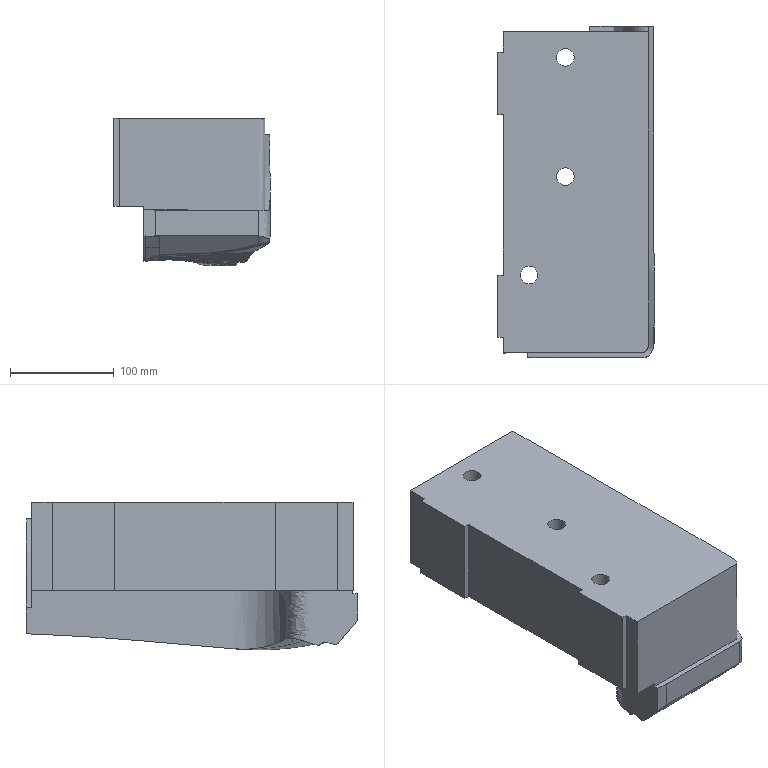Part | NX | features solid 2 | 1 solid | 172 faces | box 150.531 x 319.485 x 142.539 mm | volume 4705244 mm3 | spline 89 | cylinder 38 | plane 35 | sphere 10 | commonest cylinder face diameters 10 x9 6.001 x3 17 x3 25 x3 9 x2 11.101 x2